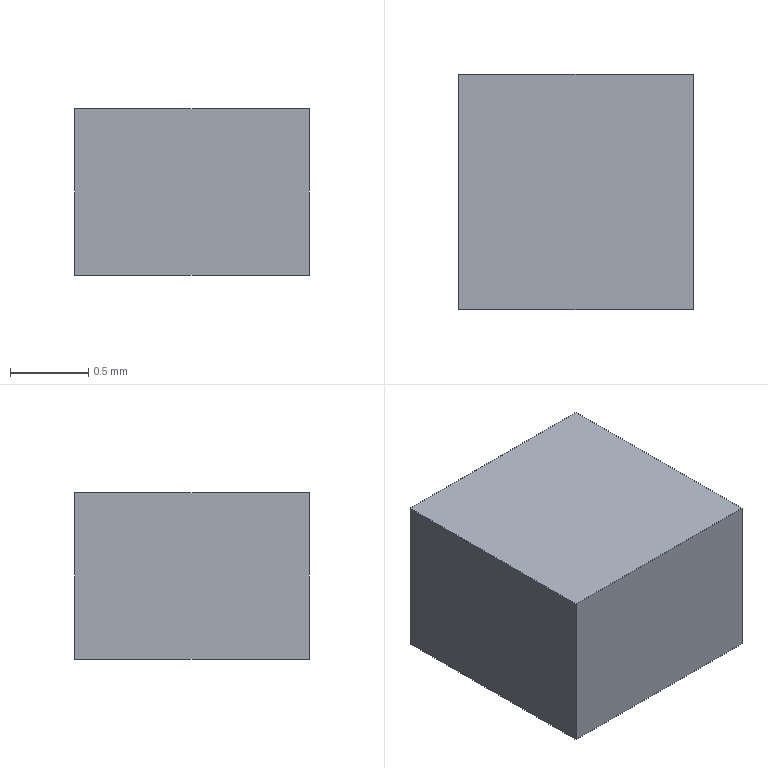Part | Creo | 1 solid | 6 faces | box 1.5 x 1.5 x 1.061 mm | volume 2.386 mm3 | plane 6
STEP:
#1=CARTESIAN_POINT('',(0.,0.,0.));
#2=DIRECTION('',(0.,0.,1.));
#3=DIRECTION('',(1.,0.,0.));
#4=AXIS2_PLACEMENT_3D('',#1,#2,#3);
#5=CARTESIAN_POINT('',(-0.75,-0.75,0.));
#6=VERTEX_POINT('',#5);
#7=CARTESIAN_POINT('',(0.75,-0.75,0.));
#8=VERTEX_POINT('',#7);
#9=CARTESIAN_POINT('',(-0.75,-0.75,0.));
#10=DIRECTION('',(1.,0.,0.));
#11=VECTOR('',#10,1.5);
#12=LINE('',#9,#11);
#13=EDGE_CURVE('',#6,#8,#12,.T.);
#14=ORIENTED_EDGE('',*,*,#13,.T.);
#15=CARTESIAN_POINT('',(0.75,0.75,0.));
#16=VERTEX_POINT('',#15);
#17=CARTESIAN_POINT('',(0.75,-0.75,0.));
#18=DIRECTION('',(0.,1.,0.));
#19=VECTOR('',#18,1.5);
#20=LINE('',#17,#19);
#21=EDGE_CURVE('',#8,#16,#20,.T.);
#22=ORIENTED_EDGE('',*,*,#21,.T.);
#23=CARTESIAN_POINT('',(-0.75,0.75,0.));
#24=VERTEX_POINT('',#23);
#25=CARTESIAN_POINT('',(0.75,0.75,0.));
#26=DIRECTION('',(-1.,0.,0.));
#27=VECTOR('',#26,1.5);
#28=LINE('',#25,#27);
#29=EDGE_CURVE('',#16,#24,#28,.T.);
#30=ORIENTED_EDGE('',*,*,#29,.T.);
#31=CARTESIAN_POINT('',(-0.75,0.75,0.));
#32=DIRECTION('',(0.,-1.,0.));
#33=VECTOR('',#32,1.5);
#34=LINE('',#31,#33);
#35=EDGE_CURVE('',#24,#6,#34,.T.);
#36=ORIENTED_EDGE('',*,*,#35,.T.);
#37=EDGE_LOOP('',(#14,#22,#30,#36));
#38=FACE_OUTER_BOUND('',#37,.F.);
#39=CARTESIAN_POINT('',(0.,0.,0.));
#40=DIRECTION('',(0.,0.,1.));
#41=DIRECTION('',(1.,0.,0.));
#42=AXIS2_PLACEMENT_3D('',#39,#40,#41);
#43=PLANE('',#42);
#44=ADVANCED_FACE('',(#38),#43,.F.);
#45=ORIENTED_EDGE('',*,*,#13,.F.);
#46=CARTESIAN_POINT('',(-0.75,-0.75,1.061));
#47=VERTEX_POINT('',#46);
#48=CARTESIAN_POINT('',(-0.75,-0.75,0.));
#49=DIRECTION('',(0.,0.,1.));
#50=VECTOR('',#49,1.061);
#51=LINE('',#48,#50);
#52=EDGE_CURVE('',#6,#47,#51,.T.);
#53=ORIENTED_EDGE('',*,*,#52,.T.);
#54=CARTESIAN_POINT('',(0.75,-0.75,1.061));
#55=VERTEX_POINT('',#54);
#56=CARTESIAN_POINT('',(-0.75,-0.75,1.061));
#57=DIRECTION('',(1.,0.,0.));
#58=VECTOR('',#57,1.5);
#59=LINE('',#56,#58);
#60=EDGE_CURVE('',#47,#55,#59,.T.);
#61=ORIENTED_EDGE('',*,*,#60,.T.);
#62=CARTESIAN_POINT('',(0.75,-0.75,0.));
#63=DIRECTION('',(0.,0.,1.));
#64=VECTOR('',#63,1.061);
#65=LINE('',#62,#64);
#66=EDGE_CURVE('',#8,#55,#65,.T.);
#67=ORIENTED_EDGE('',*,*,#66,.F.);
#68=EDGE_LOOP('',(#45,#53,#61,#67));
#69=FACE_OUTER_BOUND('',#68,.F.);
#70=CARTESIAN_POINT('',(-0.75,-0.75,0.));
#71=DIRECTION('',(0.,-1.,0.));
#72=DIRECTION('',(1.,0.,0.));
#73=AXIS2_PLACEMENT_3D('',#70,#71,#72);
#74=PLANE('',#73);
#75=ADVANCED_FACE('',(#69),#74,.T.);
#76=ORIENTED_EDGE('',*,*,#35,.F.);
#77=CARTESIAN_POINT('',(-0.75,0.75,1.061));
#78=VERTEX_POINT('',#77);
#79=CARTESIAN_POINT('',(-0.75,0.75,0.));
#80=DIRECTION('',(0.,0.,1.));
#81=VECTOR('',#80,1.061);
#82=LINE('',#79,#81);
#83=EDGE_CURVE('',#24,#78,#82,.T.);
#84=ORIENTED_EDGE('',*,*,#83,.T.);
#85=CARTESIAN_POINT('',(-0.75,0.75,1.061));
#86=DIRECTION('',(0.,-1.,0.));
#87=VECTOR('',#86,1.5);
#88=LINE('',#85,#87);
#89=EDGE_CURVE('',#78,#47,#88,.T.);
#90=ORIENTED_EDGE('',*,*,#89,.T.);
#91=ORIENTED_EDGE('',*,*,#52,.F.);
#92=EDGE_LOOP('',(#76,#84,#90,#91));
#93=FACE_OUTER_BOUND('',#92,.F.);
#94=CARTESIAN_POINT('',(-0.75,0.75,0.));
#95=DIRECTION('',(-1.,0.,0.));
#96=DIRECTION('',(0.,-1.,0.));
#97=AXIS2_PLACEMENT_3D('',#94,#95,#96);
#98=PLANE('',#97);
#99=ADVANCED_FACE('',(#93),#98,.T.);
#100=ORIENTED_EDGE('',*,*,#29,.F.);
#101=CARTESIAN_POINT('',(0.75,0.75,1.061));
#102=VERTEX_POINT('',#101);
#103=CARTESIAN_POINT('',(0.75,0.75,0.));
#104=DIRECTION('',(0.,0.,1.));
#105=VECTOR('',#104,1.061);
#106=LINE('',#103,#105);
#107=EDGE_CURVE('',#16,#102,#106,.T.);
#108=ORIENTED_EDGE('',*,*,#107,.T.);
#109=CARTESIAN_POINT('',(0.75,0.75,1.061));
#110=DIRECTION('',(-1.,0.,0.));
#111=VECTOR('',#110,1.5);
#112=LINE('',#109,#111);
#113=EDGE_CURVE('',#102,#78,#112,.T.);
#114=ORIENTED_EDGE('',*,*,#113,.T.);
#115=ORIENTED_EDGE('',*,*,#83,.F.);
#116=EDGE_LOOP('',(#100,#108,#114,#115));
#117=FACE_OUTER_BOUND('',#116,.F.);
#118=CARTESIAN_POINT('',(0.75,0.75,0.));
#119=DIRECTION('',(0.,1.,0.));
#120=DIRECTION('',(-1.,0.,0.));
#121=AXIS2_PLACEMENT_3D('',#118,#119,#120);
#122=PLANE('',#121);
#123=ADVANCED_FACE('',(#117),#122,.T.);
#124=ORIENTED_EDGE('',*,*,#21,.F.);
#125=ORIENTED_EDGE('',*,*,#66,.T.);
#126=CARTESIAN_POINT('',(0.75,-0.75,1.061));
#127=DIRECTION('',(0.,1.,0.));
#128=VECTOR('',#127,1.5);
#129=LINE('',#126,#128);
#130=EDGE_CURVE('',#55,#102,#129,.T.);
#131=ORIENTED_EDGE('',*,*,#130,.T.);
#132=ORIENTED_EDGE('',*,*,#107,.F.);
#133=EDGE_LOOP('',(#124,#125,#131,#132));
#134=FACE_OUTER_BOUND('',#133,.F.);
#135=CARTESIAN_POINT('',(0.75,-0.75,0.));
#136=DIRECTION('',(1.,0.,0.));
#137=DIRECTION('',(0.,1.,0.));
#138=AXIS2_PLACEMENT_3D('',#135,#136,#137);
#139=PLANE('',#138);
#140=ADVANCED_FACE('',(#134),#139,.T.);
#141=ORIENTED_EDGE('',*,*,#60,.F.);
#142=ORIENTED_EDGE('',*,*,#89,.F.);
#143=ORIENTED_EDGE('',*,*,#113,.F.);
#144=ORIENTED_EDGE('',*,*,#130,.F.);
#145=EDGE_LOOP('',(#141,#142,#143,#144));
#146=FACE_OUTER_BOUND('',#145,.F.);
#147=CARTESIAN_POINT('',(0.,0.,1.061));
#148=DIRECTION('',(0.,0.,1.));
#149=DIRECTION('',(1.,0.,0.));
#150=AXIS2_PLACEMENT_3D('',#147,#148,#149);
#151=PLANE('',#150);
#152=ADVANCED_FACE('',(#146),#151,.T.);
#153=CLOSED_SHELL('',(#44,#75,#99,#123,#140,#152));
#154=MANIFOLD_SOLID_BREP('',#153);
#155=(LENGTH_UNIT()NAMED_UNIT(*)SI_UNIT(.MILLI.,.METRE.));
#156=UNCERTAINTY_MEASURE_WITH_UNIT(LENGTH_MEASURE(0.0002372),#155,'','');
#157=(NAMED_UNIT(*)PLANE_ANGLE_UNIT()SI_UNIT($,.RADIAN.));
#158=PLANE_ANGLE_MEASURE_WITH_UNIT(PLANE_ANGLE_MEASURE(0.01745),#157);
#159=(CONVERSION_BASED_UNIT('DEGREE',#158)NAMED_UNIT(*)PLANE_ANGLE_UNIT());
#160=(NAMED_UNIT(*)SI_UNIT($,.STERADIAN.)SOLID_ANGLE_UNIT());
#161=(GEOMETRIC_REPRESENTATION_CONTEXT(3)GLOBAL_UNCERTAINTY_ASSIGNED_CONTEXT((#156))GLOBAL_UNIT_ASSIGNED_CONTEXT((#155,#159,#160))REPRESENTATION_CONTEXT('',''));
#162=ADVANCED_BREP_SHAPE_REPRESENTATION('',(#4,#154),#161);